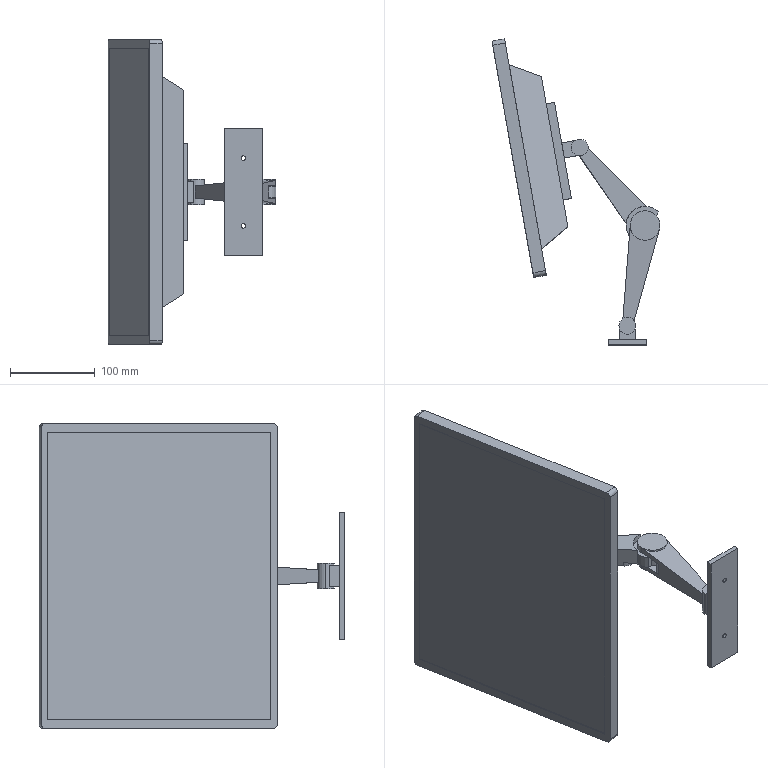Part | STEP file | TV | 5 solids | 94 faces | box 197.95 x 360.761 x 359.449 mm | volume 3578288 mm3 | plane 55 | cylinder 39 | commonest cylinder face diameters 20 x16 35 x8 45 x5 5.5 x4 10 x4 160 x2